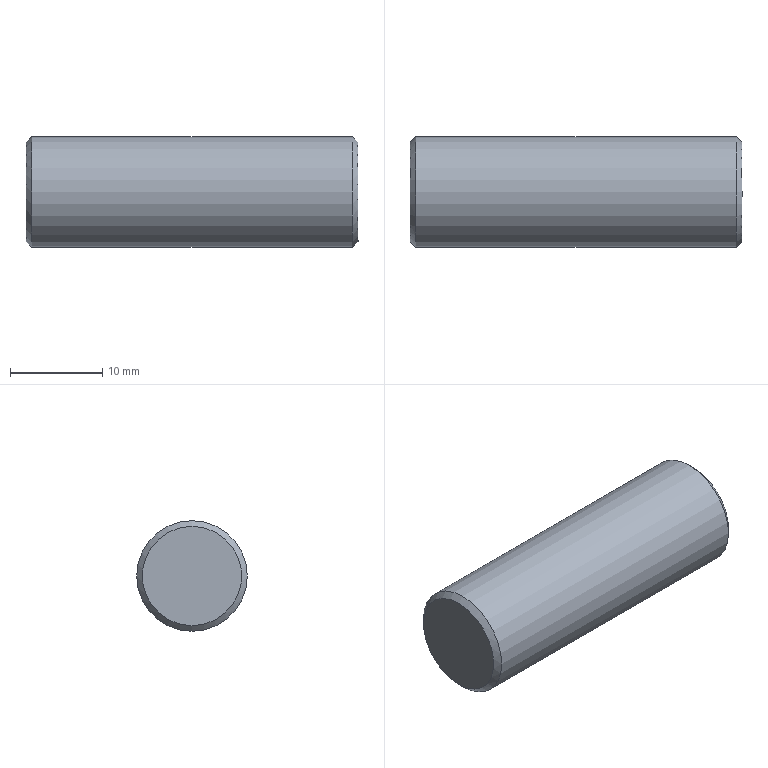Part | NX | features BREP 1 | 1 solid | 5 faces | box 36 x 12 x 12 mm | volume 4058 mm3 | cone 2 | plane 2 | cylinder 1 | commonest cylinder face diameters 12 x1
STEP:
#1=CARTESIAN_POINT('',(35.386,0.,-6.));
#2=VERTEX_POINT('',#1);
#3=CARTESIAN_POINT('',(35.386,0.,0.));
#4=DIRECTION('',(-1.,0.,0.));
#5=DIRECTION('',(0.,0.,-1.));
#6=AXIS2_PLACEMENT_3D('',#3,#4,#5);
#7=CIRCLE('',#6,6.);
#8=EDGE_CURVE('',#2,#2,#7,.T.);
#9=ORIENTED_EDGE('',*,*,#8,.T.);
#10=EDGE_LOOP('',(#9));
#11=FACE_BOUND('',#10,.T.);
#12=CARTESIAN_POINT('',(0.6135,0.,-6.));
#13=VERTEX_POINT('',#12);
#14=CARTESIAN_POINT('',(0.6135,0.,0.));
#15=DIRECTION('',(1.,0.,0.));
#16=DIRECTION('',(0.,0.,-1.));
#17=AXIS2_PLACEMENT_3D('',#14,#15,#16);
#18=CIRCLE('',#17,6.);
#19=EDGE_CURVE('',#13,#13,#18,.T.);
#20=ORIENTED_EDGE('',*,*,#19,.T.);
#21=EDGE_LOOP('',(#20));
#22=FACE_BOUND('',#21,.T.);
#23=CARTESIAN_POINT('',(36.,0.,0.));
#24=DIRECTION('',(1.,0.,0.));
#25=DIRECTION('',(0.,0.,1.));
#26=AXIS2_PLACEMENT_3D('',#23,#24,#25);
#27=CYLINDRICAL_SURFACE('',#26,6.);
#28=ADVANCED_FACE('',(#11,#22),#27,.T.);
#29=ORIENTED_EDGE('',*,*,#8,.F.);
#30=EDGE_LOOP('',(#29));
#31=FACE_BOUND('',#30,.T.);
#32=CARTESIAN_POINT('',(36.,0.,5.386));
#33=VERTEX_POINT('',#32);
#34=CARTESIAN_POINT('',(36.,0.,0.));
#35=DIRECTION('',(-1.,0.,0.));
#36=DIRECTION('',(0.,0.,1.));
#37=AXIS2_PLACEMENT_3D('',#34,#35,#36);
#38=CIRCLE('',#37,5.386);
#39=EDGE_CURVE('',#33,#33,#38,.T.);
#40=ORIENTED_EDGE('',*,*,#39,.T.);
#41=EDGE_LOOP('',(#40));
#42=FACE_BOUND('',#41,.T.);
#43=CARTESIAN_POINT('',(35.386,0.,0.));
#44=DIRECTION('',(-1.,0.,0.));
#45=DIRECTION('',(0.,0.,-1.));
#46=AXIS2_PLACEMENT_3D('',#43,#44,#45);
#47=CONICAL_SURFACE('',#46,6.,0.7854);
#48=ADVANCED_FACE('',(#31,#42),#47,.T.);
#49=ORIENTED_EDGE('',*,*,#19,.F.);
#50=EDGE_LOOP('',(#49));
#51=FACE_BOUND('',#50,.T.);
#52=CARTESIAN_POINT('',(0.,0.,-5.386));
#53=VERTEX_POINT('',#52);
#54=CARTESIAN_POINT('',(0.,0.,0.));
#55=DIRECTION('',(1.,0.,0.));
#56=DIRECTION('',(0.,0.,-1.));
#57=AXIS2_PLACEMENT_3D('',#54,#55,#56);
#58=CIRCLE('',#57,5.386);
#59=EDGE_CURVE('',#53,#53,#58,.T.);
#60=ORIENTED_EDGE('',*,*,#59,.T.);
#61=EDGE_LOOP('',(#60));
#62=FACE_BOUND('',#61,.T.);
#63=CARTESIAN_POINT('',(0.6135,0.,0.));
#64=DIRECTION('',(1.,0.,0.));
#65=DIRECTION('',(0.,0.,1.));
#66=AXIS2_PLACEMENT_3D('',#63,#64,#65);
#67=CONICAL_SURFACE('',#66,6.,0.7854);
#68=ADVANCED_FACE('',(#51,#62),#67,.T.);
#69=ORIENTED_EDGE('',*,*,#39,.F.);
#70=EDGE_LOOP('',(#69));
#71=FACE_BOUND('',#70,.T.);
#72=CARTESIAN_POINT('',(36.,5.386,0.));
#73=DIRECTION('',(-1.,0.,0.));
#74=DIRECTION('',(0.,0.,-1.));
#75=AXIS2_PLACEMENT_3D('',#72,#73,#74);
#76=PLANE('',#75);
#77=ADVANCED_FACE('',(#71),#76,.F.);
#78=ORIENTED_EDGE('',*,*,#59,.F.);
#79=EDGE_LOOP('',(#78));
#80=FACE_BOUND('',#79,.T.);
#81=CARTESIAN_POINT('',(0.,0.,0.));
#82=DIRECTION('',(1.,0.,0.));
#83=DIRECTION('',(0.,0.,1.));
#84=AXIS2_PLACEMENT_3D('',#81,#82,#83);
#85=PLANE('',#84);
#86=ADVANCED_FACE('',(#80),#85,.F.);
#87=CLOSED_SHELL('',(#28,#48,#68,#77,#86));
#88=MANIFOLD_SOLID_BREP('',#87);
#89=(LENGTH_UNIT()NAMED_UNIT(*)SI_UNIT(.MILLI.,.METRE.));
#90=UNCERTAINTY_MEASURE_WITH_UNIT(LENGTH_MEASURE(0.00001),#89,'','');
#91=(NAMED_UNIT(*)PLANE_ANGLE_UNIT()SI_UNIT($,.RADIAN.));
#92=(NAMED_UNIT(*)SI_UNIT($,.STERADIAN.)SOLID_ANGLE_UNIT());
#93=(GEOMETRIC_REPRESENTATION_CONTEXT(3)GLOBAL_UNCERTAINTY_ASSIGNED_CONTEXT((#90))GLOBAL_UNIT_ASSIGNED_CONTEXT((#89,#91,#92))REPRESENTATION_CONTEXT('',''));
#94=ADVANCED_BREP_SHAPE_REPRESENTATION('',(#88),#93);